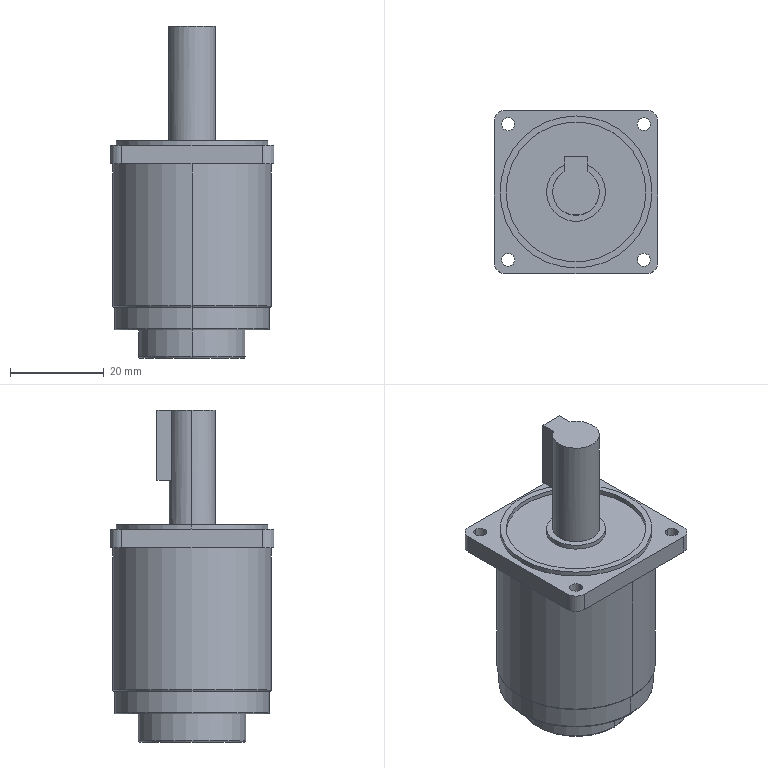Part | SolidWorks | features ICE 7, Fillet 6, Revolution 5, Attribute 3, CirPattern 2, Extrusion 2, Chamfer 1, Dome 1, Emboss 1, LibraryFeature 1, Scale 1 | 1 solid | 53 faces | box 35 x 35 x 71 mm | volume 41626 mm3 | cylinder 29 | plane 18 | torus 6 | commonest cylinder face diameters 2.75 x8 4.9 x4 10 x3 1.12 x2 12.6 x2 23 x2